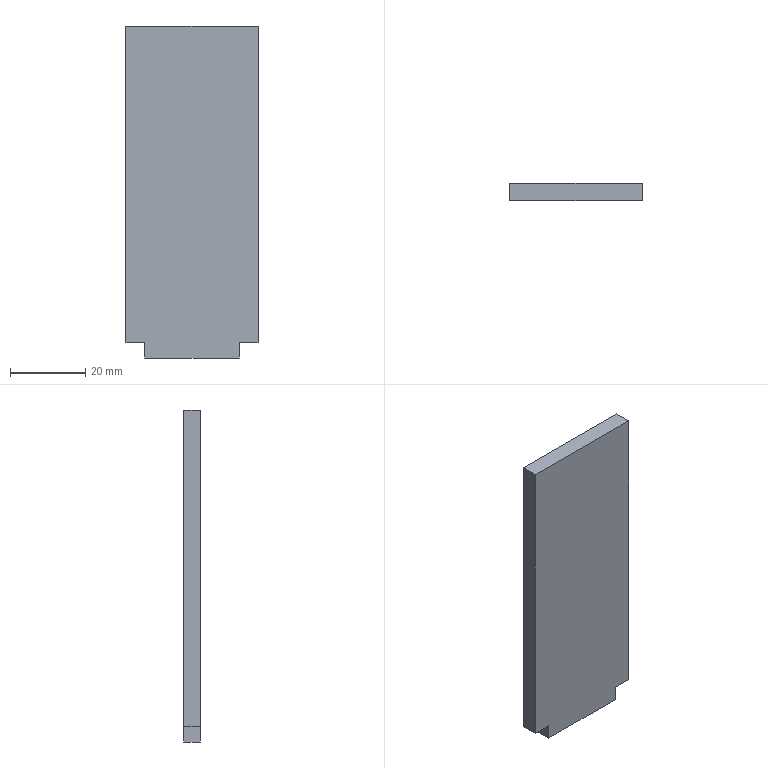Part | SolidWorks | features FlatPattern 1, SMBaseFlange 1, SheetMetal 1 | 1 solid | 10 faces | box 35 x 4.5 x 88 mm | volume 13680 mm3 | plane 10
STEP:
#1=CARTESIAN_POINT('',(17.5,0.,42.));
#2=VERTEX_POINT('',#1);
#3=CARTESIAN_POINT('',(17.5,0.,-42.));
#4=VERTEX_POINT('',#3);
#5=CARTESIAN_POINT('',(17.5,0.,-42.));
#6=DIRECTION('',(0.,0.,-1.));
#7=VECTOR('',#6,1000.);
#8=LINE('',#5,#7);
#9=EDGE_CURVE('',#2,#4,#8,.T.);
#10=ORIENTED_EDGE('',*,*,#9,.F.);
#11=CARTESIAN_POINT('',(17.5,-4.5,42.));
#12=VERTEX_POINT('',#11);
#13=CARTESIAN_POINT('',(17.5,-4.5,42.));
#14=DIRECTION('',(0.,1.,0.));
#15=VECTOR('',#14,1000.);
#16=LINE('',#13,#15);
#17=EDGE_CURVE('',#12,#2,#16,.T.);
#18=ORIENTED_EDGE('',*,*,#17,.F.);
#19=CARTESIAN_POINT('',(17.5,-4.5,-42.));
#20=VERTEX_POINT('',#19);
#21=CARTESIAN_POINT('',(17.5,-4.5,-42.));
#22=DIRECTION('',(0.,0.,-1.));
#23=VECTOR('',#22,1000.);
#24=LINE('',#21,#23);
#25=EDGE_CURVE('',#12,#20,#24,.T.);
#26=ORIENTED_EDGE('',*,*,#25,.T.);
#27=CARTESIAN_POINT('',(17.5,-4.5,-42.));
#28=DIRECTION('',(0.,1.,0.));
#29=VECTOR('',#28,1000.);
#30=LINE('',#27,#29);
#31=EDGE_CURVE('',#20,#4,#30,.T.);
#32=ORIENTED_EDGE('',*,*,#31,.T.);
#33=EDGE_LOOP('',(#10,#18,#26,#32));
#34=FACE_OUTER_BOUND('',#33,.T.);
#35=CARTESIAN_POINT('',(17.5,-4.5,-42.));
#36=DIRECTION('',(1.,0.,0.));
#37=DIRECTION('',(0.,0.,-1.));
#38=AXIS2_PLACEMENT_3D('',#35,#36,#37);
#39=PLANE('',#38);
#40=ADVANCED_FACE('',(#34),#39,.T.);
#41=CARTESIAN_POINT('',(-17.5,0.,42.));
#42=VERTEX_POINT('',#41);
#43=CARTESIAN_POINT('',(-17.5,0.,42.));
#44=DIRECTION('',(1.,0.,0.));
#45=VECTOR('',#44,1000.);
#46=LINE('',#43,#45);
#47=EDGE_CURVE('',#42,#2,#46,.T.);
#48=ORIENTED_EDGE('',*,*,#47,.F.);
#49=CARTESIAN_POINT('',(-17.5,-4.5,42.));
#50=VERTEX_POINT('',#49);
#51=CARTESIAN_POINT('',(-17.5,-4.5,42.));
#52=DIRECTION('',(0.,1.,0.));
#53=VECTOR('',#52,1000.);
#54=LINE('',#51,#53);
#55=EDGE_CURVE('',#50,#42,#54,.T.);
#56=ORIENTED_EDGE('',*,*,#55,.F.);
#57=CARTESIAN_POINT('',(-17.5,-4.5,42.));
#58=DIRECTION('',(1.,0.,0.));
#59=VECTOR('',#58,1000.);
#60=LINE('',#57,#59);
#61=EDGE_CURVE('',#50,#12,#60,.T.);
#62=ORIENTED_EDGE('',*,*,#61,.T.);
#63=ORIENTED_EDGE('',*,*,#17,.T.);
#64=EDGE_LOOP('',(#48,#56,#62,#63));
#65=FACE_OUTER_BOUND('',#64,.T.);
#66=CARTESIAN_POINT('',(-17.5,-4.5,42.));
#67=DIRECTION('',(0.,0.,1.));
#68=DIRECTION('',(1.,0.,0.));
#69=AXIS2_PLACEMENT_3D('',#66,#67,#68);
#70=PLANE('',#69);
#71=ADVANCED_FACE('',(#65),#70,.T.);
#72=CARTESIAN_POINT('',(-17.5,0.,-42.));
#73=VERTEX_POINT('',#72);
#74=CARTESIAN_POINT('',(-17.5,0.,-42.));
#75=DIRECTION('',(0.,0.,1.));
#76=VECTOR('',#75,1000.);
#77=LINE('',#74,#76);
#78=EDGE_CURVE('',#73,#42,#77,.T.);
#79=ORIENTED_EDGE('',*,*,#78,.F.);
#80=CARTESIAN_POINT('',(-17.5,-4.5,-42.));
#81=VERTEX_POINT('',#80);
#82=CARTESIAN_POINT('',(-17.5,-4.5,-42.));
#83=DIRECTION('',(0.,1.,0.));
#84=VECTOR('',#83,1000.);
#85=LINE('',#82,#84);
#86=EDGE_CURVE('',#81,#73,#85,.T.);
#87=ORIENTED_EDGE('',*,*,#86,.F.);
#88=CARTESIAN_POINT('',(-17.5,-4.5,-42.));
#89=DIRECTION('',(0.,0.,1.));
#90=VECTOR('',#89,1000.);
#91=LINE('',#88,#90);
#92=EDGE_CURVE('',#81,#50,#91,.T.);
#93=ORIENTED_EDGE('',*,*,#92,.T.);
#94=ORIENTED_EDGE('',*,*,#55,.T.);
#95=EDGE_LOOP('',(#79,#87,#93,#94));
#96=FACE_OUTER_BOUND('',#95,.T.);
#97=CARTESIAN_POINT('',(-17.5,-4.5,-42.));
#98=DIRECTION('',(-1.,0.,0.));
#99=DIRECTION('',(0.,0.,1.));
#100=AXIS2_PLACEMENT_3D('',#97,#98,#99);
#101=PLANE('',#100);
#102=ADVANCED_FACE('',(#96),#101,.T.);
#103=CARTESIAN_POINT('',(-12.5,0.,-42.));
#104=VERTEX_POINT('',#103);
#105=CARTESIAN_POINT('',(-17.5,0.,-42.));
#106=DIRECTION('',(-1.,0.,0.));
#107=VECTOR('',#106,1000.);
#108=LINE('',#105,#107);
#109=EDGE_CURVE('',#104,#73,#108,.T.);
#110=ORIENTED_EDGE('',*,*,#109,.F.);
#111=CARTESIAN_POINT('',(-12.5,-4.5,-42.));
#112=VERTEX_POINT('',#111);
#113=CARTESIAN_POINT('',(-12.5,-4.5,-42.));
#114=DIRECTION('',(0.,1.,0.));
#115=VECTOR('',#114,1000.);
#116=LINE('',#113,#115);
#117=EDGE_CURVE('',#112,#104,#116,.T.);
#118=ORIENTED_EDGE('',*,*,#117,.F.);
#119=CARTESIAN_POINT('',(-17.5,-4.5,-42.));
#120=DIRECTION('',(-1.,0.,0.));
#121=VECTOR('',#120,1000.);
#122=LINE('',#119,#121);
#123=EDGE_CURVE('',#112,#81,#122,.T.);
#124=ORIENTED_EDGE('',*,*,#123,.T.);
#125=ORIENTED_EDGE('',*,*,#86,.T.);
#126=EDGE_LOOP('',(#110,#118,#124,#125));
#127=FACE_OUTER_BOUND('',#126,.T.);
#128=CARTESIAN_POINT('',(-17.5,-4.5,-42.));
#129=DIRECTION('',(0.,0.,-1.));
#130=DIRECTION('',(-1.,0.,0.));
#131=AXIS2_PLACEMENT_3D('',#128,#129,#130);
#132=PLANE('',#131);
#133=ADVANCED_FACE('',(#127),#132,.T.);
#134=CARTESIAN_POINT('',(-12.5,0.,-46.));
#135=VERTEX_POINT('',#134);
#136=CARTESIAN_POINT('',(-12.5,0.,-42.));
#137=DIRECTION('',(0.,0.,1.));
#138=VECTOR('',#137,1000.);
#139=LINE('',#136,#138);
#140=EDGE_CURVE('',#135,#104,#139,.T.);
#141=ORIENTED_EDGE('',*,*,#140,.F.);
#142=CARTESIAN_POINT('',(-12.5,-4.5,-46.));
#143=VERTEX_POINT('',#142);
#144=CARTESIAN_POINT('',(-12.5,-4.5,-46.));
#145=DIRECTION('',(0.,1.,0.));
#146=VECTOR('',#145,1000.);
#147=LINE('',#144,#146);
#148=EDGE_CURVE('',#143,#135,#147,.T.);
#149=ORIENTED_EDGE('',*,*,#148,.F.);
#150=CARTESIAN_POINT('',(-12.5,-4.5,-42.));
#151=DIRECTION('',(0.,0.,1.));
#152=VECTOR('',#151,1000.);
#153=LINE('',#150,#152);
#154=EDGE_CURVE('',#143,#112,#153,.T.);
#155=ORIENTED_EDGE('',*,*,#154,.T.);
#156=ORIENTED_EDGE('',*,*,#117,.T.);
#157=EDGE_LOOP('',(#141,#149,#155,#156));
#158=FACE_OUTER_BOUND('',#157,.T.);
#159=CARTESIAN_POINT('',(-12.5,-4.5,-42.));
#160=DIRECTION('',(-1.,0.,0.));
#161=DIRECTION('',(0.,0.,1.));
#162=AXIS2_PLACEMENT_3D('',#159,#160,#161);
#163=PLANE('',#162);
#164=ADVANCED_FACE('',(#158),#163,.T.);
#165=CARTESIAN_POINT('',(12.5,0.,-46.));
#166=VERTEX_POINT('',#165);
#167=CARTESIAN_POINT('',(-12.5,0.,-46.));
#168=DIRECTION('',(-1.,0.,0.));
#169=VECTOR('',#168,1000.);
#170=LINE('',#167,#169);
#171=EDGE_CURVE('',#166,#135,#170,.T.);
#172=ORIENTED_EDGE('',*,*,#171,.F.);
#173=CARTESIAN_POINT('',(12.5,-4.5,-46.));
#174=VERTEX_POINT('',#173);
#175=CARTESIAN_POINT('',(12.5,-4.5,-46.));
#176=DIRECTION('',(0.,1.,0.));
#177=VECTOR('',#176,1000.);
#178=LINE('',#175,#177);
#179=EDGE_CURVE('',#174,#166,#178,.T.);
#180=ORIENTED_EDGE('',*,*,#179,.F.);
#181=CARTESIAN_POINT('',(-12.5,-4.5,-46.));
#182=DIRECTION('',(-1.,0.,0.));
#183=VECTOR('',#182,1000.);
#184=LINE('',#181,#183);
#185=EDGE_CURVE('',#174,#143,#184,.T.);
#186=ORIENTED_EDGE('',*,*,#185,.T.);
#187=ORIENTED_EDGE('',*,*,#148,.T.);
#188=EDGE_LOOP('',(#172,#180,#186,#187));
#189=FACE_OUTER_BOUND('',#188,.T.);
#190=CARTESIAN_POINT('',(-12.5,-4.5,-46.));
#191=DIRECTION('',(0.,0.,-1.));
#192=DIRECTION('',(-1.,0.,0.));
#193=AXIS2_PLACEMENT_3D('',#190,#191,#192);
#194=PLANE('',#193);
#195=ADVANCED_FACE('',(#189),#194,.T.);
#196=CARTESIAN_POINT('',(12.5,0.,-42.));
#197=VERTEX_POINT('',#196);
#198=CARTESIAN_POINT('',(12.5,0.,-46.));
#199=DIRECTION('',(0.,0.,-1.));
#200=VECTOR('',#199,1000.);
#201=LINE('',#198,#200);
#202=EDGE_CURVE('',#197,#166,#201,.T.);
#203=ORIENTED_EDGE('',*,*,#202,.F.);
#204=CARTESIAN_POINT('',(12.5,-4.5,-42.));
#205=VERTEX_POINT('',#204);
#206=CARTESIAN_POINT('',(12.5,-4.5,-42.));
#207=DIRECTION('',(0.,1.,0.));
#208=VECTOR('',#207,1000.);
#209=LINE('',#206,#208);
#210=EDGE_CURVE('',#205,#197,#209,.T.);
#211=ORIENTED_EDGE('',*,*,#210,.F.);
#212=CARTESIAN_POINT('',(12.5,-4.5,-46.));
#213=DIRECTION('',(0.,0.,-1.));
#214=VECTOR('',#213,1000.);
#215=LINE('',#212,#214);
#216=EDGE_CURVE('',#205,#174,#215,.T.);
#217=ORIENTED_EDGE('',*,*,#216,.T.);
#218=ORIENTED_EDGE('',*,*,#179,.T.);
#219=EDGE_LOOP('',(#203,#211,#217,#218));
#220=FACE_OUTER_BOUND('',#219,.T.);
#221=CARTESIAN_POINT('',(12.5,-4.5,-46.));
#222=DIRECTION('',(1.,0.,0.));
#223=DIRECTION('',(0.,0.,-1.));
#224=AXIS2_PLACEMENT_3D('',#221,#222,#223);
#225=PLANE('',#224);
#226=ADVANCED_FACE('',(#220),#225,.T.);
#227=CARTESIAN_POINT('',(12.5,0.,-42.));
#228=DIRECTION('',(-1.,0.,0.));
#229=VECTOR('',#228,1000.);
#230=LINE('',#227,#229);
#231=EDGE_CURVE('',#4,#197,#230,.T.);
#232=ORIENTED_EDGE('',*,*,#231,.F.);
#233=ORIENTED_EDGE('',*,*,#31,.F.);
#234=CARTESIAN_POINT('',(12.5,-4.5,-42.));
#235=DIRECTION('',(-1.,0.,0.));
#236=VECTOR('',#235,1000.);
#237=LINE('',#234,#236);
#238=EDGE_CURVE('',#20,#205,#237,.T.);
#239=ORIENTED_EDGE('',*,*,#238,.T.);
#240=ORIENTED_EDGE('',*,*,#210,.T.);
#241=EDGE_LOOP('',(#232,#233,#239,#240));
#242=FACE_OUTER_BOUND('',#241,.T.);
#243=CARTESIAN_POINT('',(12.5,-4.5,-42.));
#244=DIRECTION('',(0.,0.,-1.));
#245=DIRECTION('',(-1.,0.,0.));
#246=AXIS2_PLACEMENT_3D('',#243,#244,#245);
#247=PLANE('',#246);
#248=ADVANCED_FACE('',(#242),#247,.T.);
#249=ORIENTED_EDGE('',*,*,#25,.F.);
#250=ORIENTED_EDGE('',*,*,#61,.F.);
#251=ORIENTED_EDGE('',*,*,#92,.F.);
#252=ORIENTED_EDGE('',*,*,#123,.F.);
#253=ORIENTED_EDGE('',*,*,#154,.F.);
#254=ORIENTED_EDGE('',*,*,#185,.F.);
#255=ORIENTED_EDGE('',*,*,#216,.F.);
#256=ORIENTED_EDGE('',*,*,#238,.F.);
#257=EDGE_LOOP('',(#249,#250,#251,#252,#253,#254,#255,#256));
#258=FACE_OUTER_BOUND('',#257,.T.);
#259=CARTESIAN_POINT('',(0.,-4.5,0.));
#260=DIRECTION('',(0.,1.,0.));
#261=DIRECTION('',(0.,0.,1.));
#262=AXIS2_PLACEMENT_3D('',#259,#260,#261);
#263=PLANE('',#262);
#264=ADVANCED_FACE('',(#258),#263,.F.);
#265=ORIENTED_EDGE('',*,*,#9,.T.);
#266=ORIENTED_EDGE('',*,*,#231,.T.);
#267=ORIENTED_EDGE('',*,*,#202,.T.);
#268=ORIENTED_EDGE('',*,*,#171,.T.);
#269=ORIENTED_EDGE('',*,*,#140,.T.);
#270=ORIENTED_EDGE('',*,*,#109,.T.);
#271=ORIENTED_EDGE('',*,*,#78,.T.);
#272=ORIENTED_EDGE('',*,*,#47,.T.);
#273=EDGE_LOOP('',(#265,#266,#267,#268,#269,#270,#271,#272));
#274=FACE_OUTER_BOUND('',#273,.T.);
#275=CARTESIAN_POINT('',(0.,0.,0.));
#276=DIRECTION('',(0.,1.,0.));
#277=DIRECTION('',(0.,0.,1.));
#278=AXIS2_PLACEMENT_3D('',#275,#276,#277);
#279=PLANE('',#278);
#280=ADVANCED_FACE('',(#274),#279,.T.);
#281=CLOSED_SHELL('',(#40,#71,#102,#133,#164,#195,#226,#248,#264,#280));
#282=MANIFOLD_SOLID_BREP('',#281);
#283=CARTESIAN_POINT('',(0.,0.,0.));
#284=DIRECTION('',(0.,0.,1.));
#285=DIRECTION('',(1.,0.,0.));
#286=AXIS2_PLACEMENT_3D('',#283,#284,#285);
#287=(LENGTH_UNIT()NAMED_UNIT(*)SI_UNIT(.MILLI.,.METRE.));
#288=UNCERTAINTY_MEASURE_WITH_UNIT(LENGTH_MEASURE(0.00001),#287,'','');
#289=(NAMED_UNIT(*)PLANE_ANGLE_UNIT()SI_UNIT($,.RADIAN.));
#290=(NAMED_UNIT(*)SI_UNIT($,.STERADIAN.)SOLID_ANGLE_UNIT());
#291=(GEOMETRIC_REPRESENTATION_CONTEXT(3)GLOBAL_UNCERTAINTY_ASSIGNED_CONTEXT((#288))GLOBAL_UNIT_ASSIGNED_CONTEXT((#287,#289,#290))REPRESENTATION_CONTEXT('',''));
#292=ADVANCED_BREP_SHAPE_REPRESENTATION('',(#282,#286),#291);